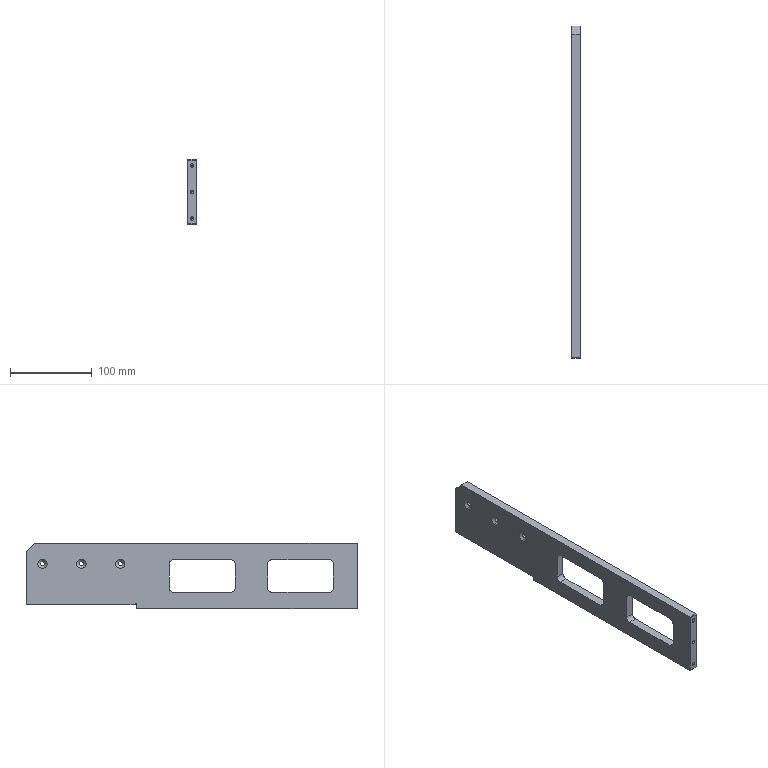Part | SolidWorks | features BaseBody 1 | 1 solid | 70 faces | box 10 x 405 x 80 mm | volume 250680 mm3 | cylinder 27 | cone 24 | plane 19 | commonest cylinder face diameters 4.2 x12 10 x8 5.5 x6 2 x1